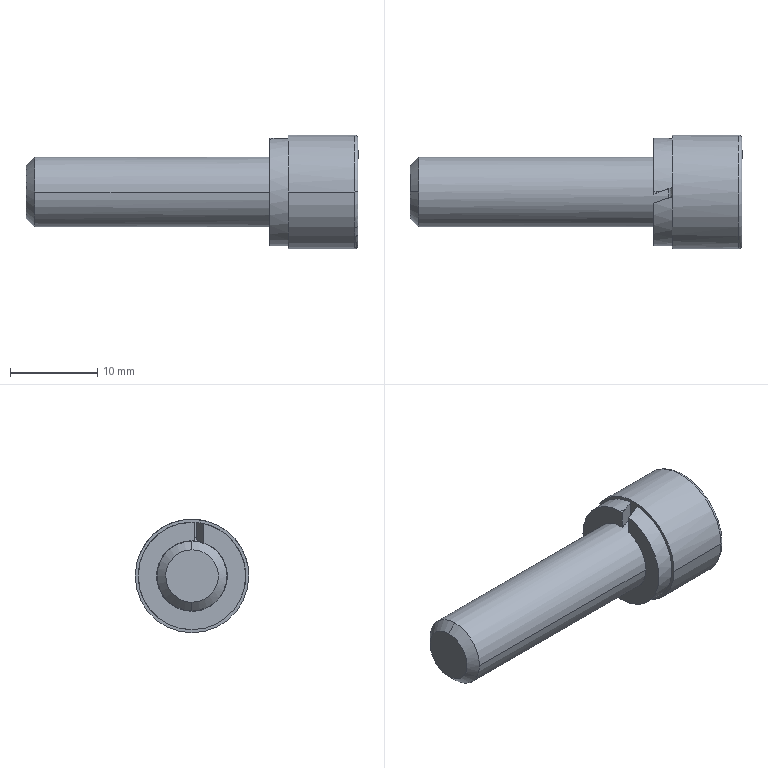Part | STEP file | Positioning_id2238_x_t | 1 solid | 29 faces | box 38 x 13 x 13 mm | volume 2572 mm3 | plane 13 | cylinder 10 | torus 4 | cone 2 | commonest cylinder face diameters 8.1 x3 12.3 x3 8 x2 13 x2